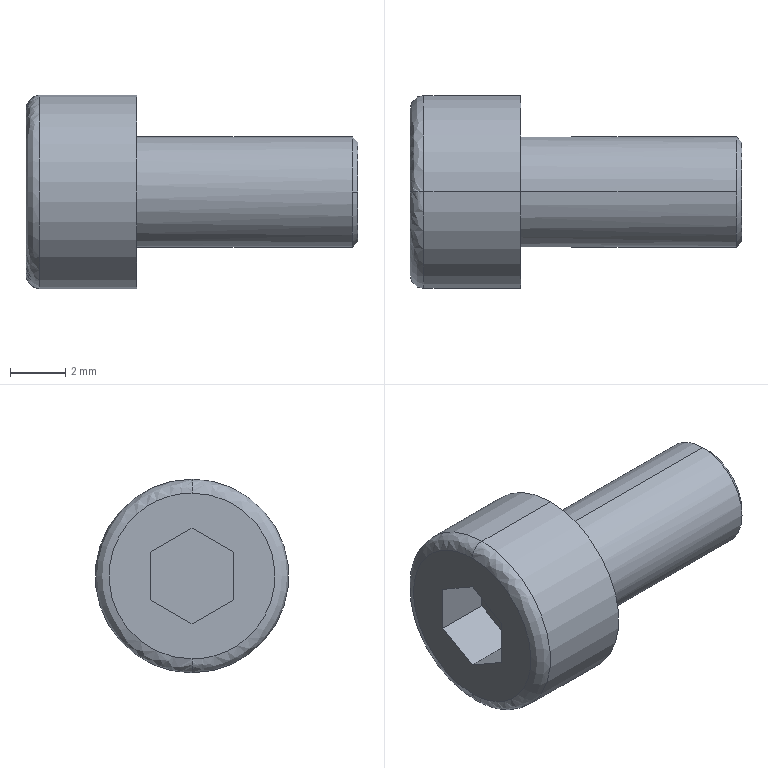Part | STEP file | Guide wheel mechanism revised.sldasm-Part-376 | 1 solid | 18 faces | box 12 x 7 x 7 mm | volume 237.501 mm3 | plane 10 | cylinder 4 | spline 2 | cone 2 | commonest cylinder face diameters 4 x2 7 x2
STEP:
#1=CARTESIAN_POINT('',(0.5,0.,3.5));
#2=VERTEX_POINT('',#1);
#3=CARTESIAN_POINT('',(0.5,0.,-3.5));
#4=VERTEX_POINT('',#3);
#5=CARTESIAN_POINT('',(0.5,0.,0.));
#6=DIRECTION('',(1.,0.,0.));
#7=DIRECTION('',(0.,0.,1.));
#8=AXIS2_PLACEMENT_3D('',#5,#6,#7);
#9=CIRCLE('',#8,3.5);
#10=EDGE_CURVE('',#2,#4,#9,.T.);
#11=ORIENTED_EDGE('',*,*,#10,.F.);
#12=CARTESIAN_POINT('',(0.,0.,3.));
#13=VERTEX_POINT('',#12);
#14=CARTESIAN_POINT('',(0.5,0.,3.));
#15=DIRECTION('',(0.,-1.,0.));
#16=DIRECTION('',(0.,0.,1.));
#17=AXIS2_PLACEMENT_3D('',#14,#15,#16);
#18=CIRCLE('',#17,0.5);
#19=EDGE_CURVE('',#2,#13,#18,.T.);
#20=ORIENTED_EDGE('',*,*,#19,.T.);
#21=CARTESIAN_POINT('',(0.,0.,-3.));
#22=VERTEX_POINT('',#21);
#23=CARTESIAN_POINT('',(0.,0.,3.));
#24=CARTESIAN_POINT('',(0.,-6.,3.));
#25=CARTESIAN_POINT('',(0.,-6.,-3.));
#26=CARTESIAN_POINT('',(0.,0.,-3.));
#27=(BOUNDED_CURVE()B_SPLINE_CURVE(3,(#23,#24,#25,#26),.UNSPECIFIED.,.F.,.F.)B_SPLINE_CURVE_WITH_KNOTS((4,4),(0.,1.),.UNSPECIFIED.)CURVE()GEOMETRIC_REPRESENTATION_ITEM()RATIONAL_B_SPLINE_CURVE((1.,0.3333,0.3333,1.))REPRESENTATION_ITEM(''));
#28=EDGE_CURVE('',#13,#22,#27,.T.);
#29=ORIENTED_EDGE('',*,*,#28,.T.);
#30=CARTESIAN_POINT('',(0.5,0.,-3.));
#31=DIRECTION('',(0.,1.,0.));
#32=DIRECTION('',(0.,0.,-1.));
#33=AXIS2_PLACEMENT_3D('',#30,#31,#32);
#34=CIRCLE('',#33,0.5);
#35=EDGE_CURVE('',#4,#22,#34,.T.);
#36=ORIENTED_EDGE('',*,*,#35,.F.);
#37=EDGE_LOOP('',(#11,#20,#29,#36));
#38=FACE_OUTER_BOUND('',#37,.T.);
#39=CARTESIAN_POINT('',(0.5,0.,3.5));
#40=CARTESIAN_POINT('',(0.5,-7.,3.5));
#41=CARTESIAN_POINT('',(0.5,-7.,-3.5));
#42=CARTESIAN_POINT('',(0.5,0.,-3.5));
#43=CARTESIAN_POINT('',(0.2071,0.,3.5));
#44=CARTESIAN_POINT('',(0.2071,-7.,3.5));
#45=CARTESIAN_POINT('',(0.2071,-7.,-3.5));
#46=CARTESIAN_POINT('',(0.2071,0.,-3.5));
#47=CARTESIAN_POINT('',(0.,0.,3.293));
#48=CARTESIAN_POINT('',(0.,-6.586,3.293));
#49=CARTESIAN_POINT('',(0.,-6.586,-3.293));
#50=CARTESIAN_POINT('',(0.,0.,-3.293));
#51=CARTESIAN_POINT('',(0.,0.,3.));
#52=CARTESIAN_POINT('',(0.,-6.,3.));
#53=CARTESIAN_POINT('',(0.,-6.,-3.));
#54=CARTESIAN_POINT('',(0.,0.,-3.));
#55=(BOUNDED_SURFACE()B_SPLINE_SURFACE(3,3,((#39,#40,#41,#42),(#43,#44,#45,#46),(#47,#48,#49,#50),(#51,#52,#53,#54)),.UNSPECIFIED.,.F.,.F.,.F.)B_SPLINE_SURFACE_WITH_KNOTS((4,4),(4,4),(0.,1.),(0.,1.),.UNSPECIFIED.)GEOMETRIC_REPRESENTATION_ITEM()RATIONAL_B_SPLINE_SURFACE(((1.,0.3333,0.3333,1.),(0.8047,0.2682,0.2682,0.8047),(0.8047,0.2682,0.2682,0.8047),(1.,0.3333,0.3333,1.)))REPRESENTATION_ITEM('')SURFACE());
#56=ADVANCED_FACE('',(#38),#55,.T.);
#57=CARTESIAN_POINT('',(11.8,2.,0.));
#58=VERTEX_POINT('',#57);
#59=CARTESIAN_POINT('',(11.8,0.,-2.));
#60=VERTEX_POINT('',#59);
#61=CARTESIAN_POINT('',(11.8,0.,0.));
#62=DIRECTION('',(-1.,0.,0.));
#63=DIRECTION('',(0.,0.,1.));
#64=AXIS2_PLACEMENT_3D('',#61,#62,#63);
#65=CIRCLE('',#64,2.);
#66=EDGE_CURVE('',#58,#60,#65,.T.);
#67=ORIENTED_EDGE('',*,*,#66,.T.);
#68=CARTESIAN_POINT('',(4.,0.,-2.));
#69=VERTEX_POINT('',#68);
#70=CARTESIAN_POINT('',(12.,0.,-2.));
#71=DIRECTION('',(-1.,0.,0.));
#72=VECTOR('',#71,1000.);
#73=LINE('',#70,#72);
#74=EDGE_CURVE('',#60,#69,#73,.T.);
#75=ORIENTED_EDGE('',*,*,#74,.T.);
#76=CARTESIAN_POINT('',(4.,0.,2.));
#77=VERTEX_POINT('',#76);
#78=CARTESIAN_POINT('',(4.,0.,0.));
#79=DIRECTION('',(1.,0.,0.));
#80=DIRECTION('',(0.,0.,1.));
#81=AXIS2_PLACEMENT_3D('',#78,#79,#80);
#82=CIRCLE('',#81,2.);
#83=EDGE_CURVE('',#69,#77,#82,.T.);
#84=ORIENTED_EDGE('',*,*,#83,.T.);
#85=CARTESIAN_POINT('',(11.8,0.,2.));
#86=VERTEX_POINT('',#85);
#87=CARTESIAN_POINT('',(12.,0.,2.));
#88=DIRECTION('',(-1.,0.,0.));
#89=VECTOR('',#88,1000.);
#90=LINE('',#87,#89);
#91=EDGE_CURVE('',#86,#77,#90,.T.);
#92=ORIENTED_EDGE('',*,*,#91,.F.);
#93=CARTESIAN_POINT('',(11.8,0.,0.));
#94=DIRECTION('',(-1.,0.,0.));
#95=DIRECTION('',(0.,0.,1.));
#96=AXIS2_PLACEMENT_3D('',#93,#94,#95);
#97=CIRCLE('',#96,2.);
#98=EDGE_CURVE('',#86,#58,#97,.T.);
#99=ORIENTED_EDGE('',*,*,#98,.T.);
#100=EDGE_LOOP('',(#67,#75,#84,#92,#99));
#101=FACE_OUTER_BOUND('',#100,.T.);
#102=CARTESIAN_POINT('',(12.,0.,0.));
#103=DIRECTION('',(-1.,0.,0.));
#104=DIRECTION('',(0.,0.,1.));
#105=AXIS2_PLACEMENT_3D('',#102,#103,#104);
#106=CYLINDRICAL_SURFACE('',#105,2.);
#107=ADVANCED_FACE('',(#101),#106,.T.);
#108=CARTESIAN_POINT('',(12.,-1.8,0.));
#109=VERTEX_POINT('',#108);
#110=CARTESIAN_POINT('',(12.,1.8,0.));
#111=VERTEX_POINT('',#110);
#112=CARTESIAN_POINT('',(12.,0.,0.));
#113=DIRECTION('',(-1.,0.,0.));
#114=DIRECTION('',(0.,-1.,0.));
#115=AXIS2_PLACEMENT_3D('',#112,#113,#114);
#116=CIRCLE('',#115,1.8);
#117=EDGE_CURVE('',#109,#111,#116,.T.);
#118=ORIENTED_EDGE('',*,*,#117,.T.);
#119=CARTESIAN_POINT('',(11.8,2.,0.));
#120=DIRECTION('',(-0.7071,0.7071,0.));
#121=VECTOR('',#120,1000.);
#122=LINE('',#119,#121);
#123=EDGE_CURVE('',#111,#58,#122,.T.);
#124=ORIENTED_EDGE('',*,*,#123,.T.);
#125=ORIENTED_EDGE('',*,*,#98,.F.);
#126=CARTESIAN_POINT('',(11.8,-2.,0.));
#127=VERTEX_POINT('',#126);
#128=CARTESIAN_POINT('',(11.8,0.,0.));
#129=DIRECTION('',(-1.,0.,0.));
#130=DIRECTION('',(0.,0.,1.));
#131=AXIS2_PLACEMENT_3D('',#128,#129,#130);
#132=CIRCLE('',#131,2.);
#133=EDGE_CURVE('',#127,#86,#132,.T.);
#134=ORIENTED_EDGE('',*,*,#133,.F.);
#135=CARTESIAN_POINT('',(11.8,-2.,0.));
#136=DIRECTION('',(-0.7071,-0.7071,0.));
#137=VECTOR('',#136,1000.);
#138=LINE('',#135,#137);
#139=EDGE_CURVE('',#109,#127,#138,.T.);
#140=ORIENTED_EDGE('',*,*,#139,.F.);
#141=EDGE_LOOP('',(#118,#124,#125,#134,#140));
#142=FACE_OUTER_BOUND('',#141,.T.);
#143=CARTESIAN_POINT('',(11.8,0.,0.));
#144=DIRECTION('',(-1.,0.,0.));
#145=DIRECTION('',(0.,-1.,0.));
#146=AXIS2_PLACEMENT_3D('',#143,#144,#145);
#147=CONICAL_SURFACE('',#146,2.,0.7854);
#148=ADVANCED_FACE('',(#142),#147,.T.);
#149=CARTESIAN_POINT('',(4.,0.,-3.5));
#150=VERTEX_POINT('',#149);
#151=CARTESIAN_POINT('',(4.,0.,3.5));
#152=VERTEX_POINT('',#151);
#153=CARTESIAN_POINT('',(4.,0.,0.));
#154=DIRECTION('',(1.,0.,0.));
#155=DIRECTION('',(0.,0.,1.));
#156=AXIS2_PLACEMENT_3D('',#153,#154,#155);
#157=CIRCLE('',#156,3.5);
#158=EDGE_CURVE('',#150,#152,#157,.T.);
#159=ORIENTED_EDGE('',*,*,#158,.F.);
#160=CARTESIAN_POINT('',(4.,0.,-3.5));
#161=DIRECTION('',(-1.,0.,0.));
#162=VECTOR('',#161,1000.);
#163=LINE('',#160,#162);
#164=EDGE_CURVE('',#150,#4,#163,.T.);
#165=ORIENTED_EDGE('',*,*,#164,.T.);
#166=CARTESIAN_POINT('',(0.5,0.,0.));
#167=DIRECTION('',(1.,0.,0.));
#168=DIRECTION('',(0.,0.,1.));
#169=AXIS2_PLACEMENT_3D('',#166,#167,#168);
#170=CIRCLE('',#169,3.5);
#171=EDGE_CURVE('',#4,#2,#170,.T.);
#172=ORIENTED_EDGE('',*,*,#171,.T.);
#173=CARTESIAN_POINT('',(4.,0.,3.5));
#174=DIRECTION('',(-1.,0.,0.));
#175=VECTOR('',#174,1000.);
#176=LINE('',#173,#175);
#177=EDGE_CURVE('',#152,#2,#176,.T.);
#178=ORIENTED_EDGE('',*,*,#177,.F.);
#179=EDGE_LOOP('',(#159,#165,#172,#178));
#180=FACE_OUTER_BOUND('',#179,.T.);
#181=CARTESIAN_POINT('',(4.,0.,0.));
#182=DIRECTION('',(-1.,0.,0.));
#183=DIRECTION('',(0.,0.,1.));
#184=AXIS2_PLACEMENT_3D('',#181,#182,#183);
#185=CYLINDRICAL_SURFACE('',#184,3.5);
#186=ADVANCED_FACE('',(#180),#185,.T.);
#187=ORIENTED_EDGE('',*,*,#74,.F.);
#188=CARTESIAN_POINT('',(11.8,0.,0.));
#189=DIRECTION('',(-1.,0.,0.));
#190=DIRECTION('',(0.,0.,1.));
#191=AXIS2_PLACEMENT_3D('',#188,#189,#190);
#192=CIRCLE('',#191,2.);
#193=EDGE_CURVE('',#60,#127,#192,.T.);
#194=ORIENTED_EDGE('',*,*,#193,.T.);
#195=ORIENTED_EDGE('',*,*,#133,.T.);
#196=ORIENTED_EDGE('',*,*,#91,.T.);
#197=CARTESIAN_POINT('',(4.,0.,0.));
#198=DIRECTION('',(1.,0.,0.));
#199=DIRECTION('',(0.,0.,1.));
#200=AXIS2_PLACEMENT_3D('',#197,#198,#199);
#201=CIRCLE('',#200,2.);
#202=EDGE_CURVE('',#77,#69,#201,.T.);
#203=ORIENTED_EDGE('',*,*,#202,.T.);
#204=EDGE_LOOP('',(#187,#194,#195,#196,#203));
#205=FACE_OUTER_BOUND('',#204,.T.);
#206=CARTESIAN_POINT('',(12.,0.,0.));
#207=DIRECTION('',(-1.,0.,0.));
#208=DIRECTION('',(0.,0.,1.));
#209=AXIS2_PLACEMENT_3D('',#206,#207,#208);
#210=CYLINDRICAL_SURFACE('',#209,2.);
#211=ADVANCED_FACE('',(#205),#210,.T.);
#212=ORIENTED_EDGE('',*,*,#202,.F.);
#213=ORIENTED_EDGE('',*,*,#83,.F.);
#214=EDGE_LOOP('',(#212,#213));
#215=FACE_BOUND('',#214,.T.);
#216=CARTESIAN_POINT('',(4.,0.,0.));
#217=DIRECTION('',(1.,0.,0.));
#218=DIRECTION('',(0.,0.,1.));
#219=AXIS2_PLACEMENT_3D('',#216,#217,#218);
#220=CIRCLE('',#219,3.5);
#221=EDGE_CURVE('',#152,#150,#220,.T.);
#222=ORIENTED_EDGE('',*,*,#221,.T.);
#223=ORIENTED_EDGE('',*,*,#158,.T.);
#224=EDGE_LOOP('',(#222,#223));
#225=FACE_OUTER_BOUND('',#224,.T.);
#226=CARTESIAN_POINT('',(4.,0.,0.));
#227=DIRECTION('',(1.,0.,0.));
#228=DIRECTION('',(0.,0.,-1.));
#229=AXIS2_PLACEMENT_3D('',#226,#227,#228);
#230=PLANE('',#229);
#231=ADVANCED_FACE('',(#215,#225),#230,.T.);
#232=ORIENTED_EDGE('',*,*,#123,.F.);
#233=CARTESIAN_POINT('',(12.,0.,0.));
#234=DIRECTION('',(-1.,0.,0.));
#235=DIRECTION('',(0.,-1.,0.));
#236=AXIS2_PLACEMENT_3D('',#233,#234,#235);
#237=CIRCLE('',#236,1.8);
#238=EDGE_CURVE('',#111,#109,#237,.T.);
#239=ORIENTED_EDGE('',*,*,#238,.T.);
#240=ORIENTED_EDGE('',*,*,#139,.T.);
#241=ORIENTED_EDGE('',*,*,#193,.F.);
#242=ORIENTED_EDGE('',*,*,#66,.F.);
#243=EDGE_LOOP('',(#232,#239,#240,#241,#242));
#244=FACE_OUTER_BOUND('',#243,.T.);
#245=CARTESIAN_POINT('',(11.8,0.,0.));
#246=DIRECTION('',(-1.,0.,0.));
#247=DIRECTION('',(0.,-1.,0.));
#248=AXIS2_PLACEMENT_3D('',#245,#246,#247);
#249=CONICAL_SURFACE('',#248,2.,0.7854);
#250=ADVANCED_FACE('',(#244),#249,.T.);
#251=ORIENTED_EDGE('',*,*,#164,.F.);
#252=ORIENTED_EDGE('',*,*,#221,.F.);
#253=ORIENTED_EDGE('',*,*,#177,.T.);
#254=ORIENTED_EDGE('',*,*,#10,.T.);
#255=EDGE_LOOP('',(#251,#252,#253,#254));
#256=FACE_OUTER_BOUND('',#255,.T.);
#257=CARTESIAN_POINT('',(4.,0.,0.));
#258=DIRECTION('',(-1.,0.,0.));
#259=DIRECTION('',(0.,0.,1.));
#260=AXIS2_PLACEMENT_3D('',#257,#258,#259);
#261=CYLINDRICAL_SURFACE('',#260,3.5);
#262=ADVANCED_FACE('',(#256),#261,.T.);
#263=ORIENTED_EDGE('',*,*,#117,.F.);
#264=ORIENTED_EDGE('',*,*,#238,.F.);
#265=EDGE_LOOP('',(#263,#264));
#266=FACE_OUTER_BOUND('',#265,.T.);
#267=CARTESIAN_POINT('',(12.,0.,0.));
#268=DIRECTION('',(1.,0.,0.));
#269=DIRECTION('',(0.,0.,-1.));
#270=AXIS2_PLACEMENT_3D('',#267,#268,#269);
#271=PLANE('',#270);
#272=ADVANCED_FACE('',(#266),#271,.T.);
#273=ORIENTED_EDGE('',*,*,#19,.F.);
#274=ORIENTED_EDGE('',*,*,#171,.F.);
#275=ORIENTED_EDGE('',*,*,#35,.T.);
#276=CARTESIAN_POINT('',(0.,0.,-3.));
#277=CARTESIAN_POINT('',(0.,6.,-3.));
#278=CARTESIAN_POINT('',(0.,6.,3.));
#279=CARTESIAN_POINT('',(0.,0.,3.));
#280=(BOUNDED_CURVE()B_SPLINE_CURVE(3,(#276,#277,#278,#279),.UNSPECIFIED.,.F.,.T.)B_SPLINE_CURVE_WITH_KNOTS((4,4),(0.,1.),.UNSPECIFIED.)CURVE()GEOMETRIC_REPRESENTATION_ITEM()RATIONAL_B_SPLINE_CURVE((1.,0.3333,0.3333,1.))REPRESENTATION_ITEM(''));
#281=EDGE_CURVE('',#22,#13,#280,.T.);
#282=ORIENTED_EDGE('',*,*,#281,.T.);
#283=EDGE_LOOP('',(#273,#274,#275,#282));
#284=FACE_OUTER_BOUND('',#283,.T.);
#285=CARTESIAN_POINT('',(0.5,0.,-3.5));
#286=CARTESIAN_POINT('',(0.5,7.,-3.5));
#287=CARTESIAN_POINT('',(0.5,7.,3.5));
#288=CARTESIAN_POINT('',(0.5,0.,3.5));
#289=CARTESIAN_POINT('',(0.2071,0.,-3.5));
#290=CARTESIAN_POINT('',(0.2071,7.,-3.5));
#291=CARTESIAN_POINT('',(0.2071,7.,3.5));
#292=CARTESIAN_POINT('',(0.2071,0.,3.5));
#293=CARTESIAN_POINT('',(0.,0.,-3.293));
#294=CARTESIAN_POINT('',(0.,6.586,-3.293));
#295=CARTESIAN_POINT('',(0.,6.586,3.293));
#296=CARTESIAN_POINT('',(0.,0.,3.293));
#297=CARTESIAN_POINT('',(0.,0.,-3.));
#298=CARTESIAN_POINT('',(0.,6.,-3.));
#299=CARTESIAN_POINT('',(0.,6.,3.));
#300=CARTESIAN_POINT('',(0.,0.,3.));
#301=(BOUNDED_SURFACE()B_SPLINE_SURFACE(3,3,((#285,#286,#287,#288),(#289,#290,#291,#292),(#293,#294,#295,#296),(#297,#298,#299,#300)),.UNSPECIFIED.,.F.,.F.,.F.)B_SPLINE_SURFACE_WITH_KNOTS((4,4),(4,4),(0.,1.),(0.,1.),.UNSPECIFIED.)GEOMETRIC_REPRESENTATION_ITEM()RATIONAL_B_SPLINE_SURFACE(((1.,0.3333,0.3333,1.),(0.8047,0.2682,0.2682,0.8047),(0.8047,0.2682,0.2682,0.8047),(1.,0.3333,0.3333,1.)))REPRESENTATION_ITEM('')SURFACE());
#302=ADVANCED_FACE('',(#284),#301,.T.);
#303=CARTESIAN_POINT('',(0.,1.5,-0.866));
#304=VERTEX_POINT('',#303);
#305=CARTESIAN_POINT('',(0.,0.,-1.732));
#306=VERTEX_POINT('',#305);
#307=CARTESIAN_POINT('',(0.,0.,-1.732));
#308=DIRECTION('',(0.,-0.866,-0.5));
#309=VECTOR('',#308,1000.);
#310=LINE('',#307,#309);
#311=EDGE_CURVE('',#304,#306,#310,.T.);
#312=ORIENTED_EDGE('',*,*,#311,.F.);
#313=CARTESIAN_POINT('',(0.,1.5,0.866));
#314=VERTEX_POINT('',#313);
#315=CARTESIAN_POINT('',(0.,1.5,-0.866));
#316=DIRECTION('',(0.,0.,-1.));
#317=VECTOR('',#316,1000.);
#318=LINE('',#315,#317);
#319=EDGE_CURVE('',#314,#304,#318,.T.);
#320=ORIENTED_EDGE('',*,*,#319,.F.);
#321=CARTESIAN_POINT('',(0.,0.,1.732));
#322=VERTEX_POINT('',#321);
#323=CARTESIAN_POINT('',(0.,1.5,0.866));
#324=DIRECTION('',(0.,0.866,-0.5));
#325=VECTOR('',#324,1000.);
#326=LINE('',#323,#325);
#327=EDGE_CURVE('',#322,#314,#326,.T.);
#328=ORIENTED_EDGE('',*,*,#327,.F.);
#329=CARTESIAN_POINT('',(0.,-1.5,0.866));
#330=VERTEX_POINT('',#329);
#331=CARTESIAN_POINT('',(0.,0.,1.732));
#332=DIRECTION('',(0.,0.866,0.5));
#333=VECTOR('',#332,1000.);
#334=LINE('',#331,#333);
#335=EDGE_CURVE('',#330,#322,#334,.T.);
#336=ORIENTED_EDGE('',*,*,#335,.F.);
#337=CARTESIAN_POINT('',(0.,-1.5,-0.866));
#338=VERTEX_POINT('',#337);
#339=CARTESIAN_POINT('',(0.,-1.5,0.866));
#340=DIRECTION('',(0.,0.,1.));
#341=VECTOR('',#340,1000.);
#342=LINE('',#339,#341);
#343=EDGE_CURVE('',#338,#330,#342,.T.);
#344=ORIENTED_EDGE('',*,*,#343,.F.);
#345=CARTESIAN_POINT('',(0.,0.,-1.732));
#346=DIRECTION('',(0.,-0.866,0.5));
#347=VECTOR('',#346,1000.);
#348=LINE('',#345,#347);
#349=EDGE_CURVE('',#306,#338,#348,.T.);
#350=ORIENTED_EDGE('',*,*,#349,.F.);
#351=EDGE_LOOP('',(#312,#320,#328,#336,#344,#350));
#352=FACE_BOUND('',#351,.T.);
#353=ORIENTED_EDGE('',*,*,#281,.F.);
#354=ORIENTED_EDGE('',*,*,#28,.F.);
#355=EDGE_LOOP('',(#353,#354));
#356=FACE_OUTER_BOUND('',#355,.T.);
#357=CARTESIAN_POINT('',(0.,0.,0.));
#358=DIRECTION('',(1.,0.,0.));
#359=DIRECTION('',(0.,0.,-1.));
#360=AXIS2_PLACEMENT_3D('',#357,#358,#359);
#361=PLANE('',#360);
#362=ADVANCED_FACE('',(#352,#356),#361,.F.);
#363=CARTESIAN_POINT('',(2.,-1.5,-0.866));
#364=VERTEX_POINT('',#363);
#365=CARTESIAN_POINT('',(2.,0.,-1.732));
#366=VERTEX_POINT('',#365);
#367=CARTESIAN_POINT('',(2.,-1.5,-0.866));
#368=DIRECTION('',(0.,0.866,-0.5));
#369=VECTOR('',#368,1000.);
#370=LINE('',#367,#369);
#371=EDGE_CURVE('',#364,#366,#370,.T.);
#372=ORIENTED_EDGE('',*,*,#371,.T.);
#373=CARTESIAN_POINT('',(2.,0.,-1.732));
#374=DIRECTION('',(-1.,0.,0.));
#375=VECTOR('',#374,1000.);
#376=LINE('',#373,#375);
#377=EDGE_CURVE('',#366,#306,#376,.T.);
#378=ORIENTED_EDGE('',*,*,#377,.T.);
#379=ORIENTED_EDGE('',*,*,#349,.T.);
#380=CARTESIAN_POINT('',(2.,-1.5,-0.866));
#381=DIRECTION('',(1.,0.,0.));
#382=VECTOR('',#381,1000.);
#383=LINE('',#380,#382);
#384=EDGE_CURVE('',#338,#364,#383,.T.);
#385=ORIENTED_EDGE('',*,*,#384,.T.);
#386=EDGE_LOOP('',(#372,#378,#379,#385));
#387=FACE_OUTER_BOUND('',#386,.T.);
#388=CARTESIAN_POINT('',(2.,-1.5,-0.866));
#389=DIRECTION('',(0.,0.5,0.866));
#390=DIRECTION('',(0.,-0.866,0.5));
#391=AXIS2_PLACEMENT_3D('',#388,#389,#390);
#392=PLANE('',#391);
#393=ADVANCED_FACE('',(#387),#392,.T.);
#394=CARTESIAN_POINT('',(2.,1.5,-0.866));
#395=VERTEX_POINT('',#394);
#396=CARTESIAN_POINT('',(2.,0.,-1.732));
#397=DIRECTION('',(0.,0.866,0.5));
#398=VECTOR('',#397,1000.);
#399=LINE('',#396,#398);
#400=EDGE_CURVE('',#366,#395,#399,.T.);
#401=ORIENTED_EDGE('',*,*,#400,.T.);
#402=CARTESIAN_POINT('',(2.,1.5,-0.866));
#403=DIRECTION('',(-1.,0.,0.));
#404=VECTOR('',#403,1000.);
#405=LINE('',#402,#404);
#406=EDGE_CURVE('',#395,#304,#405,.T.);
#407=ORIENTED_EDGE('',*,*,#406,.T.);
#408=ORIENTED_EDGE('',*,*,#311,.T.);
#409=ORIENTED_EDGE('',*,*,#377,.F.);
#410=EDGE_LOOP('',(#401,#407,#408,#409));
#411=FACE_OUTER_BOUND('',#410,.T.);
#412=CARTESIAN_POINT('',(2.,0.,-1.732));
#413=DIRECTION('',(0.,-0.5,0.866));
#414=DIRECTION('',(0.,-0.866,-0.5));
#415=AXIS2_PLACEMENT_3D('',#412,#413,#414);
#416=PLANE('',#415);
#417=ADVANCED_FACE('',(#411),#416,.T.);
#418=CARTESIAN_POINT('',(2.,-1.5,0.866));
#419=VERTEX_POINT('',#418);
#420=CARTESIAN_POINT('',(2.,-1.5,-2.598));
#421=DIRECTION('',(0.,0.,-1.));
#422=VECTOR('',#421,1000.);
#423=LINE('',#420,#422);
#424=EDGE_CURVE('',#419,#364,#423,.T.);
#425=ORIENTED_EDGE('',*,*,#424,.F.);
#426=CARTESIAN_POINT('',(2.,0.,1.732));
#427=VERTEX_POINT('',#426);
#428=CARTESIAN_POINT('',(2.,0.,1.732));
#429=DIRECTION('',(0.,-0.866,-0.5));
#430=VECTOR('',#429,1000.);
#431=LINE('',#428,#430);
#432=EDGE_CURVE('',#427,#419,#431,.T.);
#433=ORIENTED_EDGE('',*,*,#432,.F.);
#434=CARTESIAN_POINT('',(2.,1.5,0.866));
#435=VERTEX_POINT('',#434);
#436=CARTESIAN_POINT('',(2.,1.5,0.866));
#437=DIRECTION('',(0.,-0.866,0.5));
#438=VECTOR('',#437,1000.);
#439=LINE('',#436,#438);
#440=EDGE_CURVE('',#435,#427,#439,.T.);
#441=ORIENTED_EDGE('',*,*,#440,.F.);
#442=CARTESIAN_POINT('',(2.,1.5,-2.598));
#443=DIRECTION('',(0.,0.,1.));
#444=VECTOR('',#443,1000.);
#445=LINE('',#442,#444);
#446=EDGE_CURVE('',#395,#435,#445,.T.);
#447=ORIENTED_EDGE('',*,*,#446,.F.);
#448=ORIENTED_EDGE('',*,*,#400,.F.);
#449=ORIENTED_EDGE('',*,*,#371,.F.);
#450=EDGE_LOOP('',(#425,#433,#441,#447,#448,#449));
#451=FACE_OUTER_BOUND('',#450,.T.);
#452=CARTESIAN_POINT('',(2.,1.5,-2.598));
#453=DIRECTION('',(1.,0.,0.));
#454=DIRECTION('',(0.,0.,-1.));
#455=AXIS2_PLACEMENT_3D('',#452,#453,#454);
#456=PLANE('',#455);
#457=ADVANCED_FACE('',(#451),#456,.F.);
#458=ORIENTED_EDGE('',*,*,#424,.T.);
#459=ORIENTED_EDGE('',*,*,#384,.F.);
#460=ORIENTED_EDGE('',*,*,#343,.T.);
#461=CARTESIAN_POINT('',(2.,-1.5,0.866));
#462=DIRECTION('',(1.,0.,0.));
#463=VECTOR('',#462,1000.);
#464=LINE('',#461,#463);
#465=EDGE_CURVE('',#330,#419,#464,.T.);
#466=ORIENTED_EDGE('',*,*,#465,.T.);
#467=EDGE_LOOP('',(#458,#459,#460,#466));
#468=FACE_OUTER_BOUND('',#467,.T.);
#469=CARTESIAN_POINT('',(2.,-1.5,0.866));
#470=DIRECTION('',(0.,1.,0.));
#471=DIRECTION('',(0.,0.,1.));
#472=AXIS2_PLACEMENT_3D('',#469,#470,#471);
#473=PLANE('',#472);
#474=ADVANCED_FACE('',(#468),#473,.T.);
#475=ORIENTED_EDGE('',*,*,#446,.T.);
#476=CARTESIAN_POINT('',(2.,1.5,0.866));
#477=DIRECTION('',(-1.,0.,0.));
#478=VECTOR('',#477,1000.);
#479=LINE('',#476,#478);
#480=EDGE_CURVE('',#435,#314,#479,.T.);
#481=ORIENTED_EDGE('',*,*,#480,.T.);
#482=ORIENTED_EDGE('',*,*,#319,.T.);
#483=ORIENTED_EDGE('',*,*,#406,.F.);
#484=EDGE_LOOP('',(#475,#481,#482,#483));
#485=FACE_OUTER_BOUND('',#484,.T.);
#486=CARTESIAN_POINT('',(2.,1.5,-0.866));
#487=DIRECTION('',(0.,-1.,0.));
#488=DIRECTION('',(0.,0.,-1.));
#489=AXIS2_PLACEMENT_3D('',#486,#487,#488);
#490=PLANE('',#489);
#491=ADVANCED_FACE('',(#485),#490,.T.);
#492=ORIENTED_EDGE('',*,*,#432,.T.);
#493=ORIENTED_EDGE('',*,*,#465,.F.);
#494=ORIENTED_EDGE('',*,*,#335,.T.);
#495=CARTESIAN_POINT('',(2.,0.,1.732));
#496=DIRECTION('',(1.,0.,0.));
#497=VECTOR('',#496,1000.);
#498=LINE('',#495,#497);
#499=EDGE_CURVE('',#322,#427,#498,.T.);
#500=ORIENTED_EDGE('',*,*,#499,.T.);
#501=EDGE_LOOP('',(#492,#493,#494,#500));
#502=FACE_OUTER_BOUND('',#501,.T.);
#503=CARTESIAN_POINT('',(2.,0.,1.732));
#504=DIRECTION('',(0.,0.5,-0.866));
#505=DIRECTION('',(0.,0.866,0.5));
#506=AXIS2_PLACEMENT_3D('',#503,#504,#505);
#507=PLANE('',#506);
#508=ADVANCED_FACE('',(#502),#507,.T.);
#509=ORIENTED_EDGE('',*,*,#440,.T.);
#510=ORIENTED_EDGE('',*,*,#499,.F.);
#511=ORIENTED_EDGE('',*,*,#327,.T.);
#512=ORIENTED_EDGE('',*,*,#480,.F.);
#513=EDGE_LOOP('',(#509,#510,#511,#512));
#514=FACE_OUTER_BOUND('',#513,.T.);
#515=CARTESIAN_POINT('',(2.,1.5,0.866));
#516=DIRECTION('',(0.,-0.5,-0.866));
#517=DIRECTION('',(0.,0.866,-0.5));
#518=AXIS2_PLACEMENT_3D('',#515,#516,#517);
#519=PLANE('',#518);
#520=ADVANCED_FACE('',(#514),#519,.T.);
#521=CLOSED_SHELL('',(#56,#107,#148,#186,#211,#231,#250,#262,#272,#302,#362,#393,#417,#457,#474,#491,#508,#520));
#522=MANIFOLD_SOLID_BREP('',#521);
#523=CARTESIAN_POINT('',(0.,0.,0.));
#524=DIRECTION('',(0.,0.,1.));
#525=DIRECTION('',(1.,0.,0.));
#526=AXIS2_PLACEMENT_3D('',#523,#524,#525);
#527=(LENGTH_UNIT()NAMED_UNIT(*)SI_UNIT(.MILLI.,.METRE.));
#528=UNCERTAINTY_MEASURE_WITH_UNIT(LENGTH_MEASURE(0.00001),#527,'','');
#529=(NAMED_UNIT(*)PLANE_ANGLE_UNIT()SI_UNIT($,.RADIAN.));
#530=(NAMED_UNIT(*)SI_UNIT($,.STERADIAN.)SOLID_ANGLE_UNIT());
#531=(GEOMETRIC_REPRESENTATION_CONTEXT(3)GLOBAL_UNCERTAINTY_ASSIGNED_CONTEXT((#528))GLOBAL_UNIT_ASSIGNED_CONTEXT((#527,#529,#530))REPRESENTATION_CONTEXT('',''));
#532=ADVANCED_BREP_SHAPE_REPRESENTATION('',(#522,#526),#531);